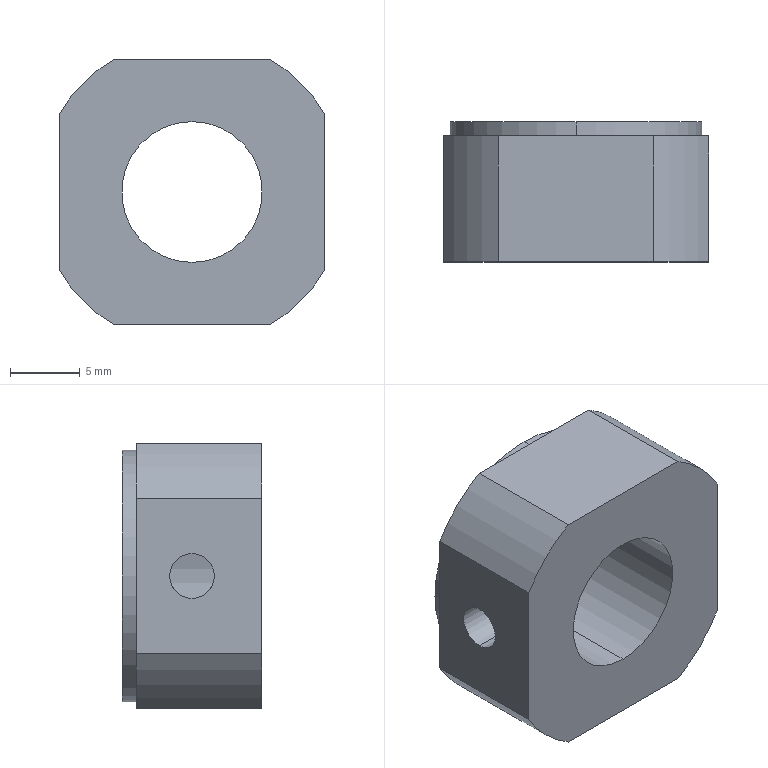Part | STEP file | SM140A-20-1140D-140A-600 Lock nut | 1 solid | 17 faces | box 19 x 10 x 19 mm | volume 2441 mm3 | cylinder 10 | plane 7 | commonest cylinder face diameters 22 x4 3.2 x2 10.05 x2 18 x2